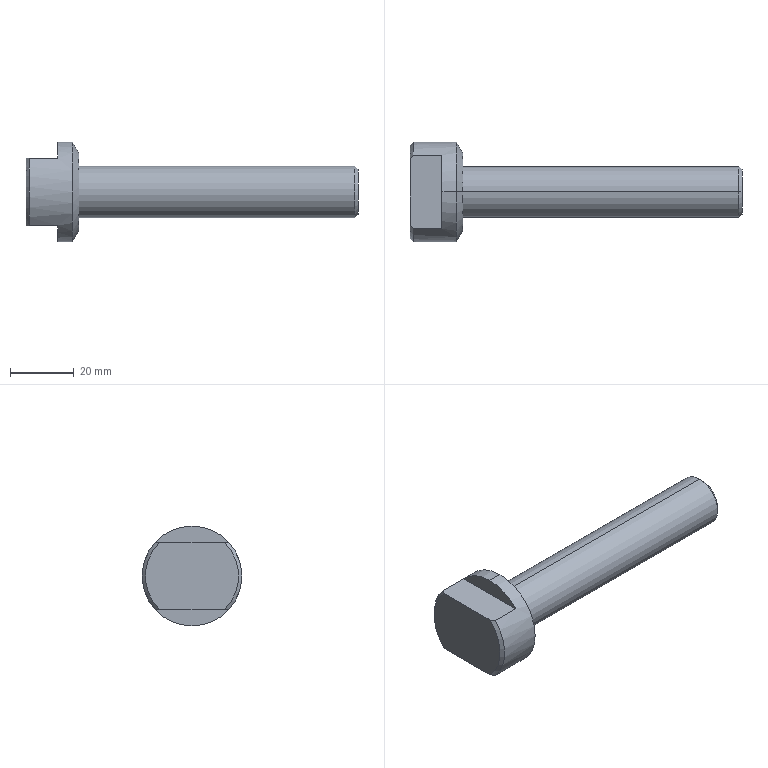Part | SolidWorks | features Chamfer 2, ICE 1, Revolution 1 | 1 solid | 17 faces | box 103.85 x 31.18 x 31.18 mm | volume 28176 mm3 | plane 7 | cone 6 | cylinder 4 | commonest cylinder face diameters 16 x2 31.18 x2
STEP:
#1=CARTESIAN_POINT('',(77.639,0.,-7.));
#2=VERTEX_POINT('',#1);
#3=CARTESIAN_POINT('',(77.639,0.,7.));
#4=VERTEX_POINT('',#3);
#5=CARTESIAN_POINT('',(77.639,0.,0.));
#6=DIRECTION('',(1.,0.,0.));
#7=DIRECTION('',(0.,0.,1.));
#8=AXIS2_PLACEMENT_3D('',#5,#6,#7);
#9=CIRCLE('',#8,7.);
#10=EDGE_CURVE('',#2,#4,#9,.T.);
#11=ORIENTED_EDGE('',*,*,#10,.F.);
#12=CARTESIAN_POINT('',(76.639,0.,-8.));
#13=VERTEX_POINT('',#12);
#14=CARTESIAN_POINT('',(76.639,0.,-8.));
#15=DIRECTION('',(-0.7071,0.,-0.7071));
#16=VECTOR('',#15,1000.);
#17=LINE('',#14,#16);
#18=EDGE_CURVE('',#2,#13,#17,.T.);
#19=ORIENTED_EDGE('',*,*,#18,.T.);
#20=CARTESIAN_POINT('',(76.639,0.,8.));
#21=VERTEX_POINT('',#20);
#22=CARTESIAN_POINT('',(76.639,0.,0.));
#23=DIRECTION('',(-1.,0.,0.));
#24=DIRECTION('',(0.,0.,1.));
#25=AXIS2_PLACEMENT_3D('',#22,#23,#24);
#26=CIRCLE('',#25,8.);
#27=EDGE_CURVE('',#21,#13,#26,.T.);
#28=ORIENTED_EDGE('',*,*,#27,.F.);
#29=CARTESIAN_POINT('',(76.639,0.,8.));
#30=DIRECTION('',(-0.7071,0.,0.7071));
#31=VECTOR('',#30,1000.);
#32=LINE('',#29,#31);
#33=EDGE_CURVE('',#4,#21,#32,.T.);
#34=ORIENTED_EDGE('',*,*,#33,.F.);
#35=EDGE_LOOP('',(#11,#19,#28,#34));
#36=FACE_OUTER_BOUND('',#35,.T.);
#37=CARTESIAN_POINT('',(76.639,0.,0.));
#38=DIRECTION('',(-1.,0.,0.));
#39=DIRECTION('',(0.,0.,1.));
#40=AXIS2_PLACEMENT_3D('',#37,#38,#39);
#41=CONICAL_SURFACE('',#40,8.,0.7854);
#42=ADVANCED_FACE('',(#36),#41,.T.);
#43=ORIENTED_EDGE('',*,*,#27,.T.);
#44=CARTESIAN_POINT('',(-9.711,0.,-8.));
#45=VERTEX_POINT('',#44);
#46=CARTESIAN_POINT('',(-41.923,0.,-8.));
#47=DIRECTION('',(-1.,0.,0.));
#48=VECTOR('',#47,1000.);
#49=LINE('',#46,#48);
#50=EDGE_CURVE('',#13,#45,#49,.T.);
#51=ORIENTED_EDGE('',*,*,#50,.T.);
#52=CARTESIAN_POINT('',(-9.711,0.,8.));
#53=VERTEX_POINT('',#52);
#54=CARTESIAN_POINT('',(-9.711,0.,0.));
#55=DIRECTION('',(-1.,0.,0.));
#56=DIRECTION('',(0.,0.,1.));
#57=AXIS2_PLACEMENT_3D('',#54,#55,#56);
#58=CIRCLE('',#57,8.);
#59=EDGE_CURVE('',#53,#45,#58,.T.);
#60=ORIENTED_EDGE('',*,*,#59,.F.);
#61=CARTESIAN_POINT('',(-41.923,0.,8.));
#62=DIRECTION('',(-1.,0.,0.));
#63=VECTOR('',#62,1000.);
#64=LINE('',#61,#63);
#65=EDGE_CURVE('',#21,#53,#64,.T.);
#66=ORIENTED_EDGE('',*,*,#65,.F.);
#67=EDGE_LOOP('',(#43,#51,#60,#66));
#68=FACE_OUTER_BOUND('',#67,.T.);
#69=CARTESIAN_POINT('',(-41.923,0.,0.));
#70=DIRECTION('',(-1.,0.,0.));
#71=DIRECTION('',(0.,0.,1.));
#72=AXIS2_PLACEMENT_3D('',#69,#70,#71);
#73=CYLINDRICAL_SURFACE('',#72,8.);
#74=ADVANCED_FACE('',(#68),#73,.T.);
#75=CARTESIAN_POINT('',(-9.711,0.,12.12));
#76=VERTEX_POINT('',#75);
#77=CARTESIAN_POINT('',(-9.711,0.,-12.12));
#78=VERTEX_POINT('',#77);
#79=CARTESIAN_POINT('',(-9.711,0.,0.));
#80=DIRECTION('',(-1.,0.,0.));
#81=DIRECTION('',(0.,0.,1.));
#82=AXIS2_PLACEMENT_3D('',#79,#80,#81);
#83=CIRCLE('',#82,12.12);
#84=EDGE_CURVE('',#76,#78,#83,.T.);
#85=ORIENTED_EDGE('',*,*,#84,.T.);
#86=CARTESIAN_POINT('',(-11.711,0.,-15.59));
#87=VERTEX_POINT('',#86);
#88=CARTESIAN_POINT('',(-9.711,0.,-12.12));
#89=DIRECTION('',(-0.4994,0.,-0.8664));
#90=VECTOR('',#89,1000.);
#91=LINE('',#88,#90);
#92=EDGE_CURVE('',#78,#87,#91,.T.);
#93=ORIENTED_EDGE('',*,*,#92,.T.);
#94=CARTESIAN_POINT('',(-11.711,0.,15.59));
#95=VERTEX_POINT('',#94);
#96=CARTESIAN_POINT('',(-11.711,0.,0.));
#97=DIRECTION('',(-1.,0.,0.));
#98=DIRECTION('',(0.,0.,1.));
#99=AXIS2_PLACEMENT_3D('',#96,#97,#98);
#100=CIRCLE('',#99,15.59);
#101=EDGE_CURVE('',#95,#87,#100,.T.);
#102=ORIENTED_EDGE('',*,*,#101,.F.);
#103=CARTESIAN_POINT('',(-9.711,0.,12.12));
#104=DIRECTION('',(-0.4994,0.,0.8664));
#105=VECTOR('',#104,1000.);
#106=LINE('',#103,#105);
#107=EDGE_CURVE('',#76,#95,#106,.T.);
#108=ORIENTED_EDGE('',*,*,#107,.F.);
#109=EDGE_LOOP('',(#85,#93,#102,#108));
#110=FACE_OUTER_BOUND('',#109,.T.);
#111=CARTESIAN_POINT('',(-9.711,0.,0.));
#112=DIRECTION('',(-1.,0.,0.));
#113=DIRECTION('',(0.,0.,1.));
#114=AXIS2_PLACEMENT_3D('',#111,#112,#113);
#115=CONICAL_SURFACE('',#114,12.12,1.048);
#116=ADVANCED_FACE('',(#110),#115,.T.);
#117=ORIENTED_EDGE('',*,*,#101,.T.);
#118=CARTESIAN_POINT('',(-16.211,0.,-15.59));
#119=VERTEX_POINT('',#118);
#120=CARTESIAN_POINT('',(-41.923,0.,-15.59));
#121=DIRECTION('',(-1.,0.,0.));
#122=VECTOR('',#121,1000.);
#123=LINE('',#120,#122);
#124=EDGE_CURVE('',#87,#119,#123,.T.);
#125=ORIENTED_EDGE('',*,*,#124,.T.);
#126=CARTESIAN_POINT('',(-16.211,11.524,-10.5));
#127=VERTEX_POINT('',#126);
#128=CARTESIAN_POINT('',(-16.211,0.,0.));
#129=DIRECTION('',(-1.,0.,0.));
#130=DIRECTION('',(0.,0.,1.));
#131=AXIS2_PLACEMENT_3D('',#128,#129,#130);
#132=CIRCLE('',#131,15.59);
#133=EDGE_CURVE('',#127,#119,#132,.T.);
#134=ORIENTED_EDGE('',*,*,#133,.F.);
#135=CARTESIAN_POINT('',(-25.211,11.524,-10.5));
#136=VERTEX_POINT('',#135);
#137=CARTESIAN_POINT('',(-41.923,11.524,-10.5));
#138=DIRECTION('',(-1.,0.,0.));
#139=VECTOR('',#138,1000.);
#140=LINE('',#137,#139);
#141=EDGE_CURVE('',#127,#136,#140,.T.);
#142=ORIENTED_EDGE('',*,*,#141,.T.);
#143=CARTESIAN_POINT('',(-25.211,11.524,10.5));
#144=VERTEX_POINT('',#143);
#145=CARTESIAN_POINT('',(-25.211,0.,0.));
#146=DIRECTION('',(1.,0.,0.));
#147=DIRECTION('',(0.,0.,-1.));
#148=AXIS2_PLACEMENT_3D('',#145,#146,#147);
#149=CIRCLE('',#148,15.59);
#150=EDGE_CURVE('',#136,#144,#149,.T.);
#151=ORIENTED_EDGE('',*,*,#150,.T.);
#152=CARTESIAN_POINT('',(-16.211,11.524,10.5));
#153=VERTEX_POINT('',#152);
#154=CARTESIAN_POINT('',(-41.923,11.524,10.5));
#155=DIRECTION('',(1.,0.,0.));
#156=VECTOR('',#155,1000.);
#157=LINE('',#154,#156);
#158=EDGE_CURVE('',#144,#153,#157,.T.);
#159=ORIENTED_EDGE('',*,*,#158,.T.);
#160=CARTESIAN_POINT('',(-16.211,0.,15.59));
#161=VERTEX_POINT('',#160);
#162=CARTESIAN_POINT('',(-16.211,0.,0.));
#163=DIRECTION('',(-1.,0.,0.));
#164=DIRECTION('',(0.,0.,1.));
#165=AXIS2_PLACEMENT_3D('',#162,#163,#164);
#166=CIRCLE('',#165,15.59);
#167=EDGE_CURVE('',#161,#153,#166,.T.);
#168=ORIENTED_EDGE('',*,*,#167,.F.);
#169=CARTESIAN_POINT('',(-41.923,0.,15.59));
#170=DIRECTION('',(-1.,0.,0.));
#171=VECTOR('',#170,1000.);
#172=LINE('',#169,#171);
#173=EDGE_CURVE('',#95,#161,#172,.T.);
#174=ORIENTED_EDGE('',*,*,#173,.F.);
#175=EDGE_LOOP('',(#117,#125,#134,#142,#151,#159,#168,#174));
#176=FACE_OUTER_BOUND('',#175,.T.);
#177=CARTESIAN_POINT('',(-41.923,0.,0.));
#178=DIRECTION('',(-1.,0.,0.));
#179=DIRECTION('',(0.,0.,1.));
#180=AXIS2_PLACEMENT_3D('',#177,#178,#179);
#181=CYLINDRICAL_SURFACE('',#180,15.59);
#182=ADVANCED_FACE('',(#176),#181,.T.);
#183=CARTESIAN_POINT('',(-26.211,10.13,10.5));
#184=VERTEX_POINT('',#183);
#185=CARTESIAN_POINT('',(-25.211,11.524,10.5));
#186=CARTESIAN_POINT('',(-25.55,11.064,10.5));
#187=CARTESIAN_POINT('',(-25.884,10.6,10.5));
#188=CARTESIAN_POINT('',(-26.211,10.13,10.5));
#189=B_SPLINE_CURVE_WITH_KNOTS('',3,(#185,#186,#187,#188),.UNSPECIFIED.,.F.,.F.,(4,4),(0.02783,0.02955),.UNSPECIFIED.);
#190=EDGE_CURVE('',#144,#184,#189,.T.);
#191=ORIENTED_EDGE('',*,*,#190,.F.);
#192=ORIENTED_EDGE('',*,*,#150,.F.);
#193=CARTESIAN_POINT('',(-26.211,10.13,-10.5));
#194=VERTEX_POINT('',#193);
#195=CARTESIAN_POINT('',(-26.211,10.13,-10.5));
#196=CARTESIAN_POINT('',(-25.884,10.6,-10.5));
#197=CARTESIAN_POINT('',(-25.55,11.064,-10.5));
#198=CARTESIAN_POINT('',(-25.211,11.524,-10.5));
#199=B_SPLINE_CURVE_WITH_KNOTS('',3,(#195,#196,#197,#198),.UNSPECIFIED.,.F.,.F.,(4,4),(0.05136,0.05308),.UNSPECIFIED.);
#200=EDGE_CURVE('',#194,#136,#199,.T.);
#201=ORIENTED_EDGE('',*,*,#200,.F.);
#202=CARTESIAN_POINT('',(-26.211,0.,0.));
#203=DIRECTION('',(-1.,0.,0.));
#204=DIRECTION('',(0.,0.,-1.));
#205=AXIS2_PLACEMENT_3D('',#202,#203,#204);
#206=CIRCLE('',#205,14.59);
#207=EDGE_CURVE('',#184,#194,#206,.T.);
#208=ORIENTED_EDGE('',*,*,#207,.F.);
#209=EDGE_LOOP('',(#191,#192,#201,#208));
#210=FACE_OUTER_BOUND('',#209,.T.);
#211=CARTESIAN_POINT('',(-26.211,0.,0.));
#212=DIRECTION('',(1.,0.,0.));
#213=DIRECTION('',(0.,0.,-1.));
#214=AXIS2_PLACEMENT_3D('',#211,#212,#213);
#215=CONICAL_SURFACE('',#214,14.59,0.7854);
#216=ADVANCED_FACE('',(#210),#215,.T.);
#217=CARTESIAN_POINT('',(-26.211,-10.13,-10.5));
#218=VERTEX_POINT('',#217);
#219=CARTESIAN_POINT('',(-26.211,-10.13,10.5));
#220=VERTEX_POINT('',#219);
#221=CARTESIAN_POINT('',(-26.211,0.,0.));
#222=DIRECTION('',(-1.,0.,0.));
#223=DIRECTION('',(0.,0.,-1.));
#224=AXIS2_PLACEMENT_3D('',#221,#222,#223);
#225=CIRCLE('',#224,14.59);
#226=EDGE_CURVE('',#218,#220,#225,.T.);
#227=ORIENTED_EDGE('',*,*,#226,.T.);
#228=CARTESIAN_POINT('',(-26.211,15.561,10.5));
#229=DIRECTION('',(0.,-1.,0.));
#230=VECTOR('',#229,1000.);
#231=LINE('',#228,#230);
#232=EDGE_CURVE('',#184,#220,#231,.T.);
#233=ORIENTED_EDGE('',*,*,#232,.F.);
#234=ORIENTED_EDGE('',*,*,#207,.T.);
#235=CARTESIAN_POINT('',(-26.211,45.255,-10.5));
#236=DIRECTION('',(0.,1.,0.));
#237=VECTOR('',#236,1000.);
#238=LINE('',#235,#237);
#239=EDGE_CURVE('',#218,#194,#238,.T.);
#240=ORIENTED_EDGE('',*,*,#239,.F.);
#241=EDGE_LOOP('',(#227,#233,#234,#240));
#242=FACE_OUTER_BOUND('',#241,.T.);
#243=CARTESIAN_POINT('',(-26.211,0.,0.));
#244=DIRECTION('',(1.,0.,0.));
#245=DIRECTION('',(0.,0.,-1.));
#246=AXIS2_PLACEMENT_3D('',#243,#244,#245);
#247=PLANE('',#246);
#248=ADVANCED_FACE('',(#242),#247,.F.);
#249=ORIENTED_EDGE('',*,*,#124,.F.);
#250=CARTESIAN_POINT('',(-11.711,0.,0.));
#251=DIRECTION('',(-1.,0.,0.));
#252=DIRECTION('',(0.,0.,1.));
#253=AXIS2_PLACEMENT_3D('',#250,#251,#252);
#254=CIRCLE('',#253,15.59);
#255=EDGE_CURVE('',#87,#95,#254,.T.);
#256=ORIENTED_EDGE('',*,*,#255,.T.);
#257=ORIENTED_EDGE('',*,*,#173,.T.);
#258=CARTESIAN_POINT('',(-16.211,-11.524,10.5));
#259=VERTEX_POINT('',#258);
#260=CARTESIAN_POINT('',(-16.211,0.,0.));
#261=DIRECTION('',(-1.,0.,0.));
#262=DIRECTION('',(0.,0.,1.));
#263=AXIS2_PLACEMENT_3D('',#260,#261,#262);
#264=CIRCLE('',#263,15.59);
#265=EDGE_CURVE('',#259,#161,#264,.T.);
#266=ORIENTED_EDGE('',*,*,#265,.F.);
#267=CARTESIAN_POINT('',(-25.211,-11.524,10.5));
#268=VERTEX_POINT('',#267);
#269=CARTESIAN_POINT('',(-41.923,-11.524,10.5));
#270=DIRECTION('',(-1.,0.,0.));
#271=VECTOR('',#270,1000.);
#272=LINE('',#269,#271);
#273=EDGE_CURVE('',#259,#268,#272,.T.);
#274=ORIENTED_EDGE('',*,*,#273,.T.);
#275=CARTESIAN_POINT('',(-25.211,-11.524,-10.5));
#276=VERTEX_POINT('',#275);
#277=CARTESIAN_POINT('',(-25.211,0.,0.));
#278=DIRECTION('',(1.,0.,0.));
#279=DIRECTION('',(0.,0.,-1.));
#280=AXIS2_PLACEMENT_3D('',#277,#278,#279);
#281=CIRCLE('',#280,15.59);
#282=EDGE_CURVE('',#268,#276,#281,.T.);
#283=ORIENTED_EDGE('',*,*,#282,.T.);
#284=CARTESIAN_POINT('',(-16.211,-11.524,-10.5));
#285=VERTEX_POINT('',#284);
#286=CARTESIAN_POINT('',(-41.923,-11.524,-10.5));
#287=DIRECTION('',(1.,0.,0.));
#288=VECTOR('',#287,1000.);
#289=LINE('',#286,#288);
#290=EDGE_CURVE('',#276,#285,#289,.T.);
#291=ORIENTED_EDGE('',*,*,#290,.T.);
#292=CARTESIAN_POINT('',(-16.211,0.,0.));
#293=DIRECTION('',(-1.,0.,0.));
#294=DIRECTION('',(0.,0.,1.));
#295=AXIS2_PLACEMENT_3D('',#292,#293,#294);
#296=CIRCLE('',#295,15.59);
#297=EDGE_CURVE('',#119,#285,#296,.T.);
#298=ORIENTED_EDGE('',*,*,#297,.F.);
#299=EDGE_LOOP('',(#249,#256,#257,#266,#274,#283,#291,#298));
#300=FACE_OUTER_BOUND('',#299,.T.);
#301=CARTESIAN_POINT('',(-41.923,0.,0.));
#302=DIRECTION('',(-1.,0.,0.));
#303=DIRECTION('',(0.,0.,1.));
#304=AXIS2_PLACEMENT_3D('',#301,#302,#303);
#305=CYLINDRICAL_SURFACE('',#304,15.59);
#306=ADVANCED_FACE('',(#300),#305,.T.);
#307=ORIENTED_EDGE('',*,*,#92,.F.);
#308=CARTESIAN_POINT('',(-9.711,0.,0.));
#309=DIRECTION('',(-1.,0.,0.));
#310=DIRECTION('',(0.,0.,1.));
#311=AXIS2_PLACEMENT_3D('',#308,#309,#310);
#312=CIRCLE('',#311,12.12);
#313=EDGE_CURVE('',#78,#76,#312,.T.);
#314=ORIENTED_EDGE('',*,*,#313,.T.);
#315=ORIENTED_EDGE('',*,*,#107,.T.);
#316=ORIENTED_EDGE('',*,*,#255,.F.);
#317=EDGE_LOOP('',(#307,#314,#315,#316));
#318=FACE_OUTER_BOUND('',#317,.T.);
#319=CARTESIAN_POINT('',(-9.711,0.,0.));
#320=DIRECTION('',(-1.,0.,0.));
#321=DIRECTION('',(0.,0.,1.));
#322=AXIS2_PLACEMENT_3D('',#319,#320,#321);
#323=CONICAL_SURFACE('',#322,12.12,1.048);
#324=ADVANCED_FACE('',(#318),#323,.T.);
#325=ORIENTED_EDGE('',*,*,#84,.F.);
#326=ORIENTED_EDGE('',*,*,#313,.F.);
#327=EDGE_LOOP('',(#325,#326));
#328=FACE_OUTER_BOUND('',#327,.T.);
#329=ORIENTED_EDGE('',*,*,#59,.T.);
#330=CARTESIAN_POINT('',(-9.711,0.,0.));
#331=DIRECTION('',(-1.,0.,0.));
#332=DIRECTION('',(0.,0.,1.));
#333=AXIS2_PLACEMENT_3D('',#330,#331,#332);
#334=CIRCLE('',#333,8.);
#335=EDGE_CURVE('',#45,#53,#334,.T.);
#336=ORIENTED_EDGE('',*,*,#335,.T.);
#337=EDGE_LOOP('',(#329,#336));
#338=FACE_BOUND('',#337,.T.);
#339=CARTESIAN_POINT('',(-9.711,12.12,0.));
#340=DIRECTION('',(-1.,0.,0.));
#341=DIRECTION('',(0.,0.,1.));
#342=AXIS2_PLACEMENT_3D('',#339,#340,#341);
#343=PLANE('',#342);
#344=ADVANCED_FACE('',(#328,#338),#343,.F.);
#345=ORIENTED_EDGE('',*,*,#50,.F.);
#346=CARTESIAN_POINT('',(76.639,0.,0.));
#347=DIRECTION('',(-1.,0.,0.));
#348=DIRECTION('',(0.,0.,1.));
#349=AXIS2_PLACEMENT_3D('',#346,#347,#348);
#350=CIRCLE('',#349,8.);
#351=EDGE_CURVE('',#13,#21,#350,.T.);
#352=ORIENTED_EDGE('',*,*,#351,.T.);
#353=ORIENTED_EDGE('',*,*,#65,.T.);
#354=ORIENTED_EDGE('',*,*,#335,.F.);
#355=EDGE_LOOP('',(#345,#352,#353,#354));
#356=FACE_OUTER_BOUND('',#355,.T.);
#357=CARTESIAN_POINT('',(-41.923,0.,0.));
#358=DIRECTION('',(-1.,0.,0.));
#359=DIRECTION('',(0.,0.,1.));
#360=AXIS2_PLACEMENT_3D('',#357,#358,#359);
#361=CYLINDRICAL_SURFACE('',#360,8.);
#362=ADVANCED_FACE('',(#356),#361,.T.);
#363=CARTESIAN_POINT('',(77.639,0.,0.));
#364=DIRECTION('',(1.,0.,0.));
#365=DIRECTION('',(0.,0.,1.));
#366=AXIS2_PLACEMENT_3D('',#363,#364,#365);
#367=CIRCLE('',#366,7.);
#368=EDGE_CURVE('',#4,#2,#367,.T.);
#369=ORIENTED_EDGE('',*,*,#368,.T.);
#370=ORIENTED_EDGE('',*,*,#10,.T.);
#371=EDGE_LOOP('',(#369,#370));
#372=FACE_OUTER_BOUND('',#371,.T.);
#373=CARTESIAN_POINT('',(77.639,8.,0.));
#374=DIRECTION('',(-1.,0.,0.));
#375=DIRECTION('',(0.,0.,1.));
#376=AXIS2_PLACEMENT_3D('',#373,#374,#375);
#377=PLANE('',#376);
#378=ADVANCED_FACE('',(#372),#377,.F.);
#379=CARTESIAN_POINT('',(-26.211,-10.13,10.5));
#380=CARTESIAN_POINT('',(-25.885,-10.6,10.5));
#381=CARTESIAN_POINT('',(-25.551,-11.064,10.5));
#382=CARTESIAN_POINT('',(-25.211,-11.524,10.5));
#383=B_SPLINE_CURVE_WITH_KNOTS('',3,(#379,#380,#381,#382),.UNSPECIFIED.,.F.,.F.,(4,4),(0.0517,0.05342),.UNSPECIFIED.);
#384=EDGE_CURVE('',#220,#268,#383,.T.);
#385=ORIENTED_EDGE('',*,*,#384,.F.);
#386=ORIENTED_EDGE('',*,*,#226,.F.);
#387=CARTESIAN_POINT('',(-25.211,-11.524,-10.5));
#388=CARTESIAN_POINT('',(-25.551,-11.064,-10.5));
#389=CARTESIAN_POINT('',(-25.884,-10.6,-10.5));
#390=CARTESIAN_POINT('',(-26.211,-10.13,-10.5));
#391=B_SPLINE_CURVE_WITH_KNOTS('',3,(#387,#388,#389,#390),.UNSPECIFIED.,.F.,.F.,(4,4),(0.02752,0.02924),.UNSPECIFIED.);
#392=EDGE_CURVE('',#276,#218,#391,.T.);
#393=ORIENTED_EDGE('',*,*,#392,.F.);
#394=ORIENTED_EDGE('',*,*,#282,.F.);
#395=EDGE_LOOP('',(#385,#386,#393,#394));
#396=FACE_OUTER_BOUND('',#395,.T.);
#397=CARTESIAN_POINT('',(-26.211,0.,0.));
#398=DIRECTION('',(1.,0.,0.));
#399=DIRECTION('',(0.,0.,-1.));
#400=AXIS2_PLACEMENT_3D('',#397,#398,#399);
#401=CONICAL_SURFACE('',#400,14.59,0.7854);
#402=ADVANCED_FACE('',(#396),#401,.T.);
#403=ORIENTED_EDGE('',*,*,#18,.F.);
#404=ORIENTED_EDGE('',*,*,#368,.F.);
#405=ORIENTED_EDGE('',*,*,#33,.T.);
#406=ORIENTED_EDGE('',*,*,#351,.F.);
#407=EDGE_LOOP('',(#403,#404,#405,#406));
#408=FACE_OUTER_BOUND('',#407,.T.);
#409=CARTESIAN_POINT('',(76.639,0.,0.));
#410=DIRECTION('',(-1.,0.,0.));
#411=DIRECTION('',(0.,0.,1.));
#412=AXIS2_PLACEMENT_3D('',#409,#410,#411);
#413=CONICAL_SURFACE('',#412,8.,0.7854);
#414=ADVANCED_FACE('',(#408),#413,.T.);
#415=ORIENTED_EDGE('',*,*,#133,.T.);
#416=ORIENTED_EDGE('',*,*,#297,.T.);
#417=CARTESIAN_POINT('',(-16.211,45.255,-10.5));
#418=DIRECTION('',(0.,1.,0.));
#419=VECTOR('',#418,1000.);
#420=LINE('',#417,#419);
#421=EDGE_CURVE('',#285,#127,#420,.T.);
#422=ORIENTED_EDGE('',*,*,#421,.T.);
#423=EDGE_LOOP('',(#415,#416,#422));
#424=FACE_OUTER_BOUND('',#423,.T.);
#425=CARTESIAN_POINT('',(-16.211,0.,0.));
#426=DIRECTION('',(-1.,0.,0.));
#427=DIRECTION('',(0.,0.,1.));
#428=AXIS2_PLACEMENT_3D('',#425,#426,#427);
#429=PLANE('',#428);
#430=ADVANCED_FACE('',(#424),#429,.T.);
#431=ORIENTED_EDGE('',*,*,#392,.T.);
#432=ORIENTED_EDGE('',*,*,#239,.T.);
#433=ORIENTED_EDGE('',*,*,#200,.T.);
#434=ORIENTED_EDGE('',*,*,#141,.F.);
#435=ORIENTED_EDGE('',*,*,#421,.F.);
#436=ORIENTED_EDGE('',*,*,#290,.F.);
#437=EDGE_LOOP('',(#431,#432,#433,#434,#435,#436));
#438=FACE_OUTER_BOUND('',#437,.T.);
#439=CARTESIAN_POINT('',(-16.211,45.255,-10.5));
#440=DIRECTION('',(0.,0.,1.));
#441=DIRECTION('',(0.,-1.,0.));
#442=AXIS2_PLACEMENT_3D('',#439,#440,#441);
#443=PLANE('',#442);
#444=ADVANCED_FACE('',(#438),#443,.F.);
#445=ORIENTED_EDGE('',*,*,#265,.T.);
#446=ORIENTED_EDGE('',*,*,#167,.T.);
#447=CARTESIAN_POINT('',(-16.211,15.561,10.5));
#448=DIRECTION('',(0.,-1.,0.));
#449=VECTOR('',#448,1000.);
#450=LINE('',#447,#449);
#451=EDGE_CURVE('',#153,#259,#450,.T.);
#452=ORIENTED_EDGE('',*,*,#451,.T.);
#453=EDGE_LOOP('',(#445,#446,#452));
#454=FACE_OUTER_BOUND('',#453,.T.);
#455=CARTESIAN_POINT('',(-16.211,0.,0.));
#456=DIRECTION('',(-1.,0.,0.));
#457=DIRECTION('',(0.,0.,1.));
#458=AXIS2_PLACEMENT_3D('',#455,#456,#457);
#459=PLANE('',#458);
#460=ADVANCED_FACE('',(#454),#459,.T.);
#461=ORIENTED_EDGE('',*,*,#190,.T.);
#462=ORIENTED_EDGE('',*,*,#232,.T.);
#463=ORIENTED_EDGE('',*,*,#384,.T.);
#464=ORIENTED_EDGE('',*,*,#273,.F.);
#465=ORIENTED_EDGE('',*,*,#451,.F.);
#466=ORIENTED_EDGE('',*,*,#158,.F.);
#467=EDGE_LOOP('',(#461,#462,#463,#464,#465,#466));
#468=FACE_OUTER_BOUND('',#467,.T.);
#469=CARTESIAN_POINT('',(-16.211,15.561,10.5));
#470=DIRECTION('',(0.,0.,-1.));
#471=DIRECTION('',(0.,1.,0.));
#472=AXIS2_PLACEMENT_3D('',#469,#470,#471);
#473=PLANE('',#472);
#474=ADVANCED_FACE('',(#468),#473,.F.);
#475=CLOSED_SHELL('',(#42,#74,#116,#182,#216,#248,#306,#324,#344,#362,#378,#402,#414,#430,#444,#460,#474));
#476=MANIFOLD_SOLID_BREP('',#475);
#477=CARTESIAN_POINT('',(0.,0.,0.));
#478=DIRECTION('',(0.,0.,1.));
#479=DIRECTION('',(1.,0.,0.));
#480=AXIS2_PLACEMENT_3D('',#477,#478,#479);
#481=(LENGTH_UNIT()NAMED_UNIT(*)SI_UNIT(.MILLI.,.METRE.));
#482=UNCERTAINTY_MEASURE_WITH_UNIT(LENGTH_MEASURE(0.00001),#481,'','');
#483=(NAMED_UNIT(*)PLANE_ANGLE_UNIT()SI_UNIT($,.RADIAN.));
#484=(NAMED_UNIT(*)SI_UNIT($,.STERADIAN.)SOLID_ANGLE_UNIT());
#485=(GEOMETRIC_REPRESENTATION_CONTEXT(3)GLOBAL_UNCERTAINTY_ASSIGNED_CONTEXT((#482))GLOBAL_UNIT_ASSIGNED_CONTEXT((#481,#483,#484))REPRESENTATION_CONTEXT('',''));
#486=ADVANCED_BREP_SHAPE_REPRESENTATION('',(#476,#480),#485);